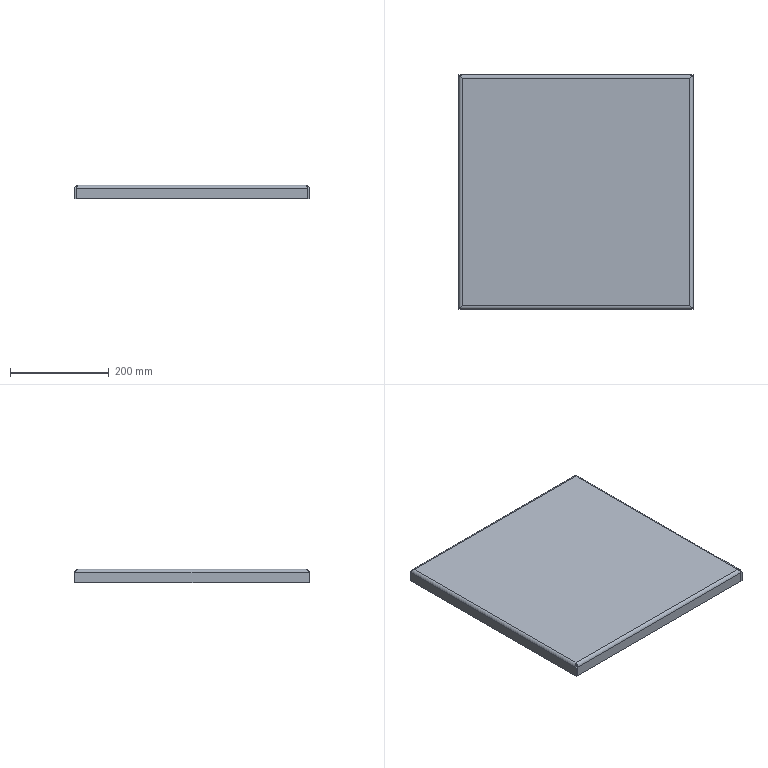Part | SolidWorks | features CornerFeat 4, FlatPattern 1, SMBaseFlange 1, SMMiteredFlange 1, SheetMetal 1 | 1 solid | 38 faces | box 476 x 476 x 28 mm | volume 807964 mm3 | plane 22 | spline 8 | cylinder 8 | commonest cylinder face diameters 8 x4 14 x4
STEP:
#1=CARTESIAN_POINT('',(231.,-231.,0.));
#2=VERTEX_POINT('',#1);
#3=CARTESIAN_POINT('',(-231.,-231.,0.));
#4=VERTEX_POINT('',#3);
#5=CARTESIAN_POINT('',(2585.,-231.,0.));
#6=DIRECTION('',(-1.,0.,0.));
#7=VECTOR('',#6,1000.);
#8=LINE('',#5,#7);
#9=EDGE_CURVE('',#2,#4,#8,.T.);
#10=ORIENTED_EDGE('',*,*,#9,.F.);
#11=CARTESIAN_POINT('',(231.,231.,0.));
#12=VERTEX_POINT('',#11);
#13=CARTESIAN_POINT('',(231.,2585.,0.));
#14=DIRECTION('',(0.,-1.,0.));
#15=VECTOR('',#14,1000.);
#16=LINE('',#13,#15);
#17=EDGE_CURVE('',#12,#2,#16,.T.);
#18=ORIENTED_EDGE('',*,*,#17,.F.);
#19=CARTESIAN_POINT('',(-231.,231.,0.));
#20=VERTEX_POINT('',#19);
#21=CARTESIAN_POINT('',(-2585.,231.,0.));
#22=DIRECTION('',(1.,0.,0.));
#23=VECTOR('',#22,1000.);
#24=LINE('',#21,#23);
#25=EDGE_CURVE('',#20,#12,#24,.T.);
#26=ORIENTED_EDGE('',*,*,#25,.F.);
#27=CARTESIAN_POINT('',(-231.,-2585.,0.));
#28=DIRECTION('',(0.,1.,0.));
#29=VECTOR('',#28,1000.);
#30=LINE('',#27,#29);
#31=EDGE_CURVE('',#4,#20,#30,.T.);
#32=ORIENTED_EDGE('',*,*,#31,.F.);
#33=EDGE_LOOP('',(#10,#18,#26,#32));
#34=FACE_OUTER_BOUND('',#33,.T.);
#35=CARTESIAN_POINT('',(0.,0.,0.));
#36=DIRECTION('',(0.,0.,-1.));
#37=DIRECTION('',(-1.,0.,0.));
#38=AXIS2_PLACEMENT_3D('',#35,#36,#37);
#39=PLANE('',#38);
#40=ADVANCED_FACE('',(#34),#39,.F.);
#41=CARTESIAN_POINT('',(231.,231.,-3.));
#42=VERTEX_POINT('',#41);
#43=CARTESIAN_POINT('',(231.,-231.,-3.));
#44=VERTEX_POINT('',#43);
#45=CARTESIAN_POINT('',(231.,2585.,-3.));
#46=DIRECTION('',(0.,-1.,0.));
#47=VECTOR('',#46,1000.);
#48=LINE('',#45,#47);
#49=EDGE_CURVE('',#42,#44,#48,.T.);
#50=ORIENTED_EDGE('',*,*,#49,.T.);
#51=CARTESIAN_POINT('',(-231.,-231.,-3.));
#52=VERTEX_POINT('',#51);
#53=CARTESIAN_POINT('',(2585.,-231.,-3.));
#54=DIRECTION('',(-1.,0.,0.));
#55=VECTOR('',#54,1000.);
#56=LINE('',#53,#55);
#57=EDGE_CURVE('',#44,#52,#56,.T.);
#58=ORIENTED_EDGE('',*,*,#57,.T.);
#59=CARTESIAN_POINT('',(-231.,231.,-3.));
#60=VERTEX_POINT('',#59);
#61=CARTESIAN_POINT('',(-231.,-2585.,-3.));
#62=DIRECTION('',(0.,1.,0.));
#63=VECTOR('',#62,1000.);
#64=LINE('',#61,#63);
#65=EDGE_CURVE('',#52,#60,#64,.T.);
#66=ORIENTED_EDGE('',*,*,#65,.T.);
#67=CARTESIAN_POINT('',(-2585.,231.,-3.));
#68=DIRECTION('',(1.,0.,0.));
#69=VECTOR('',#68,1000.);
#70=LINE('',#67,#69);
#71=EDGE_CURVE('',#60,#42,#70,.T.);
#72=ORIENTED_EDGE('',*,*,#71,.T.);
#73=EDGE_LOOP('',(#50,#58,#66,#72));
#74=FACE_OUTER_BOUND('',#73,.T.);
#75=CARTESIAN_POINT('',(0.,0.,-3.));
#76=DIRECTION('',(0.,0.,-1.));
#77=DIRECTION('',(-1.,0.,0.));
#78=AXIS2_PLACEMENT_3D('',#75,#76,#77);
#79=PLANE('',#78);
#80=ADVANCED_FACE('',(#74),#79,.T.);
#81=CARTESIAN_POINT('',(234.9,235.,-7.));
#82=VERTEX_POINT('',#81);
#83=CARTESIAN_POINT('',(234.9,238.,-7.));
#84=VERTEX_POINT('',#83);
#85=CARTESIAN_POINT('',(234.9,235.,-7.));
#86=CARTESIAN_POINT('',(234.9,238.,-7.));
#87=B_SPLINE_CURVE_WITH_KNOTS('',1,(#85,#86),.UNSPECIFIED.,.F.,.F.,(2,2),(0.,1.),.UNSPECIFIED.);
#88=EDGE_CURVE('',#82,#84,#87,.T.);
#89=ORIENTED_EDGE('',*,*,#88,.T.);
#90=CARTESIAN_POINT('',(234.9,238.,-7.));
#91=CARTESIAN_POINT('',(234.736,238.,-6.538));
#92=CARTESIAN_POINT('',(234.575,237.955,-6.083));
#93=CARTESIAN_POINT('',(234.332,237.821,-5.412));
#94=CARTESIAN_POINT('',(234.251,237.766,-5.191));
#95=CARTESIAN_POINT('',(234.089,237.633,-4.752));
#96=CARTESIAN_POINT('',(234.007,237.555,-4.534));
#97=CARTESIAN_POINT('',(233.762,237.291,-3.897));
#98=CARTESIAN_POINT('',(233.601,237.076,-3.494));
#99=CARTESIAN_POINT('',(233.358,236.696,-2.925));
#100=CARTESIAN_POINT('',(233.277,236.56,-2.741));
#101=CARTESIAN_POINT('',(233.114,236.268,-2.385));
#102=CARTESIAN_POINT('',(233.032,236.113,-2.213));
#103=CARTESIAN_POINT('',(232.788,235.627,-1.727));
#104=CARTESIAN_POINT('',(232.627,235.275,-1.438));
#105=CARTESIAN_POINT('',(232.303,234.515,-0.9293));
#106=CARTESIAN_POINT('',(232.138,234.104,-0.7093));
#107=CARTESIAN_POINT('',(231.814,233.26,-0.3593));
#108=CARTESIAN_POINT('',(231.653,232.824,-0.2263));
#109=CARTESIAN_POINT('',(231.328,231.925,-0.04623));
#110=CARTESIAN_POINT('',(231.164,231.462,0.));
#111=CARTESIAN_POINT('',(231.,231.,0.));
#112=B_SPLINE_CURVE_WITH_KNOTS('',3,(#90,#91,#92,#93,#94,#95,#96,#97,#98,#99,#100,#101,#102,#103,#104,#105,#106,#107,#108,#109,#110,#111),.UNSPECIFIED.,.F.,.F.,(4,2,2,2,2,2,2,2,2,2,4),(0.,0.00145,0.002176,0.002901,0.004351,0.005076,0.005802,0.007252,0.008702,0.01015,0.0116),.UNSPECIFIED.);
#113=EDGE_CURVE('',#84,#12,#112,.T.);
#114=ORIENTED_EDGE('',*,*,#113,.T.);
#115=CARTESIAN_POINT('',(231.,231.,-3.));
#116=CARTESIAN_POINT('',(231.,231.,0.));
#117=B_SPLINE_CURVE_WITH_KNOTS('',1,(#115,#116),.UNSPECIFIED.,.F.,.F.,(2,2),(0.,1.),.UNSPECIFIED.);
#118=EDGE_CURVE('',#42,#12,#117,.T.);
#119=ORIENTED_EDGE('',*,*,#118,.F.);
#120=CARTESIAN_POINT('',(234.9,235.,-7.));
#121=CARTESIAN_POINT('',(234.736,235.,-6.736));
#122=CARTESIAN_POINT('',(234.574,234.974,-6.475));
#123=CARTESIAN_POINT('',(234.249,234.872,-5.962));
#124=CARTESIAN_POINT('',(234.085,234.794,-5.707));
#125=CARTESIAN_POINT('',(233.76,234.594,-5.224));
#126=CARTESIAN_POINT('',(233.599,234.47,-4.994));
#127=CARTESIAN_POINT('',(233.275,234.181,-4.56));
#128=CARTESIAN_POINT('',(233.111,234.012,-4.355));
#129=CARTESIAN_POINT('',(232.786,233.641,-3.985));
#130=CARTESIAN_POINT('',(232.625,233.44,-3.819));
#131=CARTESIAN_POINT('',(232.301,233.006,-3.53));
#132=CARTESIAN_POINT('',(232.137,232.772,-3.404));
#133=CARTESIAN_POINT('',(231.812,232.288,-3.204));
#134=CARTESIAN_POINT('',(231.651,232.038,-3.128));
#135=CARTESIAN_POINT('',(231.327,231.527,-3.026));
#136=CARTESIAN_POINT('',(231.164,231.264,-3.));
#137=CARTESIAN_POINT('',(231.,231.,-3.));
#138=B_SPLINE_CURVE_WITH_KNOTS('',3,(#120,#121,#122,#123,#124,#125,#126,#127,#128,#129,#130,#131,#132,#133,#134,#135,#136,#137),.UNSPECIFIED.,.F.,.F.,(4,2,2,2,2,2,2,2,4),(0.,0.0009235,0.001847,0.00277,0.003694,0.004617,0.005541,0.006464,0.007388),.UNSPECIFIED.);
#139=EDGE_CURVE('',#82,#42,#138,.T.);
#140=ORIENTED_EDGE('',*,*,#139,.F.);
#141=EDGE_LOOP('',(#89,#114,#119,#140));
#142=FACE_OUTER_BOUND('',#141,.T.);
#143=CARTESIAN_POINT('',(234.9,238.03,-7.));
#144=CARTESIAN_POINT('',(234.575,238.03,-6.08));
#145=CARTESIAN_POINT('',(234.25,237.847,-5.16));
#146=CARTESIAN_POINT('',(233.6,237.143,-3.459));
#147=CARTESIAN_POINT('',(233.275,236.622,-2.68));
#148=CARTESIAN_POINT('',(232.625,235.32,-1.378));
#149=CARTESIAN_POINT('',(232.3,234.541,-0.857));
#150=CARTESIAN_POINT('',(231.65,232.84,-0.1527));
#151=CARTESIAN_POINT('',(231.325,231.92,0.0303));
#152=CARTESIAN_POINT('',(231.,231.,0.0303));
#153=CARTESIAN_POINT('',(234.9,238.,-7.));
#154=CARTESIAN_POINT('',(234.575,238.,-6.084));
#155=CARTESIAN_POINT('',(234.25,237.818,-5.168));
#156=CARTESIAN_POINT('',(233.6,237.117,-3.475));
#157=CARTESIAN_POINT('',(233.275,236.598,-2.698));
#158=CARTESIAN_POINT('',(232.625,235.302,-1.402));
#159=CARTESIAN_POINT('',(232.3,234.525,-0.8835));
#160=CARTESIAN_POINT('',(231.65,232.832,-0.1822));
#161=CARTESIAN_POINT('',(231.325,231.916,0.));
#162=CARTESIAN_POINT('',(231.,231.,0.));
#163=CARTESIAN_POINT('',(234.9,235.,-7.));
#164=CARTESIAN_POINT('',(234.575,235.,-6.476));
#165=CARTESIAN_POINT('',(234.25,234.896,-5.953));
#166=CARTESIAN_POINT('',(233.6,234.495,-4.986));
#167=CARTESIAN_POINT('',(233.275,234.199,-4.542));
#168=CARTESIAN_POINT('',(232.625,233.458,-3.801));
#169=CARTESIAN_POINT('',(232.3,233.014,-3.505));
#170=CARTESIAN_POINT('',(231.65,232.047,-3.104));
#171=CARTESIAN_POINT('',(231.325,231.524,-3.));
#172=CARTESIAN_POINT('',(231.,231.,-3.));
#173=CARTESIAN_POINT('',(234.9,234.97,-7.));
#174=CARTESIAN_POINT('',(234.575,234.97,-6.48));
#175=CARTESIAN_POINT('',(234.25,234.867,-5.961));
#176=CARTESIAN_POINT('',(233.6,234.469,-5.001));
#177=CARTESIAN_POINT('',(233.275,234.175,-4.56));
#178=CARTESIAN_POINT('',(232.625,233.44,-3.825));
#179=CARTESIAN_POINT('',(232.3,232.999,-3.531));
#180=CARTESIAN_POINT('',(231.65,232.039,-3.133));
#181=CARTESIAN_POINT('',(231.325,231.52,-3.03));
#182=CARTESIAN_POINT('',(231.,231.,-3.03));
#183=B_SPLINE_SURFACE_WITH_KNOTS('',1,3,((#143,#144,#145,#146,#147,#148,#149,#150,#151,#152),(#153,#154,#155,#156,#157,#158,#159,#160,#161,#162),(#163,#164,#165,#166,#167,#168,#169,#170,#171,#172),(#173,#174,#175,#176,#177,#178,#179,#180,#181,#182)),.UNSPECIFIED.,.F.,.F.,.F.,(2,1,1,2),(4,2,2,2,4),(-0.0101,0.,1.,1.01),(0.,0.25,0.5,0.75,1.),.UNSPECIFIED.);
#184=ADVANCED_FACE('',(#142),#183,.F.);
#185=CARTESIAN_POINT('',(-234.9,238.,-7.));
#186=VERTEX_POINT('',#185);
#187=CARTESIAN_POINT('',(-231.,231.,0.));
#188=CARTESIAN_POINT('',(-231.164,231.462,0.));
#189=CARTESIAN_POINT('',(-231.325,231.917,-0.04539));
#190=CARTESIAN_POINT('',(-231.568,232.588,-0.1786));
#191=CARTESIAN_POINT('',(-231.649,232.809,-0.2339));
#192=CARTESIAN_POINT('',(-231.811,233.248,-0.3668));
#193=CARTESIAN_POINT('',(-231.893,233.466,-0.4447));
#194=CARTESIAN_POINT('',(-232.138,234.103,-0.7087));
#195=CARTESIAN_POINT('',(-232.299,234.506,-0.924));
#196=CARTESIAN_POINT('',(-232.542,235.075,-1.304));
#197=CARTESIAN_POINT('',(-232.623,235.259,-1.44));
#198=CARTESIAN_POINT('',(-232.786,235.615,-1.732));
#199=CARTESIAN_POINT('',(-232.868,235.787,-1.887));
#200=CARTESIAN_POINT('',(-233.112,236.273,-2.373));
#201=CARTESIAN_POINT('',(-233.273,236.562,-2.725));
#202=CARTESIAN_POINT('',(-233.597,237.071,-3.485));
#203=CARTESIAN_POINT('',(-233.762,237.291,-3.896));
#204=CARTESIAN_POINT('',(-234.086,237.641,-4.74));
#205=CARTESIAN_POINT('',(-234.247,237.774,-5.176));
#206=CARTESIAN_POINT('',(-234.572,237.954,-6.075));
#207=CARTESIAN_POINT('',(-234.736,238.,-6.538));
#208=CARTESIAN_POINT('',(-234.9,238.,-7.));
#209=B_SPLINE_CURVE_WITH_KNOTS('',3,(#187,#188,#189,#190,#191,#192,#193,#194,#195,#196,#197,#198,#199,#200,#201,#202,#203,#204,#205,#206,#207,#208),.UNSPECIFIED.,.F.,.F.,(4,2,2,2,2,2,2,2,2,2,4),(0.,0.00145,0.002176,0.002901,0.004351,0.005076,0.005802,0.007252,0.008702,0.01015,0.0116),.UNSPECIFIED.);
#210=EDGE_CURVE('',#20,#186,#209,.T.);
#211=ORIENTED_EDGE('',*,*,#210,.T.);
#212=CARTESIAN_POINT('',(-234.9,235.,-7.));
#213=VERTEX_POINT('',#212);
#214=CARTESIAN_POINT('',(-234.9,235.,-7.));
#215=CARTESIAN_POINT('',(-234.9,236.,-7.));
#216=CARTESIAN_POINT('',(-234.9,237.,-7.));
#217=CARTESIAN_POINT('',(-234.9,238.,-7.));
#218=B_SPLINE_CURVE_WITH_KNOTS('',3,(#214,#215,#216,#217),.UNSPECIFIED.,.F.,.F.,(4,4),(0.,1.),.UNSPECIFIED.);
#219=EDGE_CURVE('',#213,#186,#218,.T.);
#220=ORIENTED_EDGE('',*,*,#219,.F.);
#221=CARTESIAN_POINT('',(-231.,231.,-3.));
#222=CARTESIAN_POINT('',(-231.164,231.264,-3.));
#223=CARTESIAN_POINT('',(-231.326,231.525,-3.026));
#224=CARTESIAN_POINT('',(-231.651,232.038,-3.128));
#225=CARTESIAN_POINT('',(-231.815,232.292,-3.205));
#226=CARTESIAN_POINT('',(-232.14,232.776,-3.406));
#227=CARTESIAN_POINT('',(-232.301,233.006,-3.53));
#228=CARTESIAN_POINT('',(-232.625,233.44,-3.819));
#229=CARTESIAN_POINT('',(-232.789,233.645,-3.988));
#230=CARTESIAN_POINT('',(-233.114,234.015,-4.359));
#231=CARTESIAN_POINT('',(-233.275,234.181,-4.561));
#232=CARTESIAN_POINT('',(-233.599,234.47,-4.994));
#233=CARTESIAN_POINT('',(-233.763,234.596,-5.228));
#234=CARTESIAN_POINT('',(-234.088,234.796,-5.712));
#235=CARTESIAN_POINT('',(-234.25,234.872,-5.962));
#236=CARTESIAN_POINT('',(-234.573,234.974,-6.473));
#237=CARTESIAN_POINT('',(-234.736,235.,-6.736));
#238=CARTESIAN_POINT('',(-234.9,235.,-7.));
#239=B_SPLINE_CURVE_WITH_KNOTS('',3,(#221,#222,#223,#224,#225,#226,#227,#228,#229,#230,#231,#232,#233,#234,#235,#236,#237,#238),.UNSPECIFIED.,.F.,.F.,(4,2,2,2,2,2,2,2,4),(0.,0.0009233,0.001847,0.00277,0.003693,0.004617,0.00554,0.006463,0.007387),.UNSPECIFIED.);
#240=EDGE_CURVE('',#60,#213,#239,.T.);
#241=ORIENTED_EDGE('',*,*,#240,.F.);
#242=CARTESIAN_POINT('',(-231.,231.,-3.));
#243=CARTESIAN_POINT('',(-231.,231.,0.));
#244=B_SPLINE_CURVE_WITH_KNOTS('',1,(#242,#243),.UNSPECIFIED.,.F.,.F.,(2,2),(0.,1.),.UNSPECIFIED.);
#245=EDGE_CURVE('',#60,#20,#244,.T.);
#246=ORIENTED_EDGE('',*,*,#245,.T.);
#247=EDGE_LOOP('',(#211,#220,#241,#246));
#248=FACE_OUTER_BOUND('',#247,.T.);
#249=CARTESIAN_POINT('',(-231.,231.,0.03));
#250=CARTESIAN_POINT('',(-231.325,231.92,0.03));
#251=CARTESIAN_POINT('',(-231.65,232.84,-0.153));
#252=CARTESIAN_POINT('',(-232.3,234.54,-0.8573));
#253=CARTESIAN_POINT('',(-232.625,235.32,-1.378));
#254=CARTESIAN_POINT('',(-233.275,236.622,-2.68));
#255=CARTESIAN_POINT('',(-233.6,237.143,-3.46));
#256=CARTESIAN_POINT('',(-234.25,237.847,-5.16));
#257=CARTESIAN_POINT('',(-234.575,238.03,-6.08));
#258=CARTESIAN_POINT('',(-234.9,238.03,-7.));
#259=CARTESIAN_POINT('',(-231.,231.,0.));
#260=CARTESIAN_POINT('',(-231.325,231.916,0.));
#261=CARTESIAN_POINT('',(-231.65,232.832,-0.1822));
#262=CARTESIAN_POINT('',(-232.3,234.525,-0.8835));
#263=CARTESIAN_POINT('',(-232.625,235.302,-1.402));
#264=CARTESIAN_POINT('',(-233.275,236.598,-2.698));
#265=CARTESIAN_POINT('',(-233.6,237.117,-3.475));
#266=CARTESIAN_POINT('',(-234.25,237.818,-5.168));
#267=CARTESIAN_POINT('',(-234.575,238.,-6.084));
#268=CARTESIAN_POINT('',(-234.9,238.,-7.));
#269=CARTESIAN_POINT('',(-231.,231.,-3.));
#270=CARTESIAN_POINT('',(-231.325,231.524,-3.));
#271=CARTESIAN_POINT('',(-231.65,232.047,-3.104));
#272=CARTESIAN_POINT('',(-232.3,233.014,-3.505));
#273=CARTESIAN_POINT('',(-232.625,233.458,-3.801));
#274=CARTESIAN_POINT('',(-233.275,234.199,-4.542));
#275=CARTESIAN_POINT('',(-233.6,234.495,-4.986));
#276=CARTESIAN_POINT('',(-234.25,234.896,-5.953));
#277=CARTESIAN_POINT('',(-234.575,235.,-6.476));
#278=CARTESIAN_POINT('',(-234.9,235.,-7.));
#279=CARTESIAN_POINT('',(-231.,231.,-3.03));
#280=CARTESIAN_POINT('',(-231.325,231.52,-3.03));
#281=CARTESIAN_POINT('',(-231.65,232.039,-3.134));
#282=CARTESIAN_POINT('',(-232.3,232.999,-3.531));
#283=CARTESIAN_POINT('',(-232.625,233.44,-3.826));
#284=CARTESIAN_POINT('',(-233.275,234.174,-4.56));
#285=CARTESIAN_POINT('',(-233.6,234.469,-5.001));
#286=CARTESIAN_POINT('',(-234.25,234.866,-5.961));
#287=CARTESIAN_POINT('',(-234.575,234.97,-6.48));
#288=CARTESIAN_POINT('',(-234.9,234.97,-7.));
#289=B_SPLINE_SURFACE_WITH_KNOTS('',1,3,((#249,#250,#251,#252,#253,#254,#255,#256,#257,#258),(#259,#260,#261,#262,#263,#264,#265,#266,#267,#268),(#269,#270,#271,#272,#273,#274,#275,#276,#277,#278),(#279,#280,#281,#282,#283,#284,#285,#286,#287,#288)),.UNSPECIFIED.,.F.,.F.,.F.,(2,1,1,2),(4,2,2,2,4),(-0.01,0.,1.,1.01),(0.,0.25,0.5,0.75,1.),.UNSPECIFIED.);
#290=ADVANCED_FACE('',(#248),#289,.F.);
#291=ORIENTED_EDGE('',*,*,#71,.F.);
#292=ORIENTED_EDGE('',*,*,#240,.T.);
#293=CARTESIAN_POINT('',(-2585.,235.,-7.));
#294=DIRECTION('',(1.,0.,0.));
#295=VECTOR('',#294,1000.);
#296=LINE('',#293,#295);
#297=EDGE_CURVE('',#213,#82,#296,.T.);
#298=ORIENTED_EDGE('',*,*,#297,.T.);
#299=ORIENTED_EDGE('',*,*,#139,.T.);
#300=EDGE_LOOP('',(#291,#292,#298,#299));
#301=FACE_OUTER_BOUND('',#300,.T.);
#302=CARTESIAN_POINT('',(-469.889,231.,-7.));
#303=DIRECTION('',(1.,0.,0.));
#304=DIRECTION('',(0.,1.,0.));
#305=AXIS2_PLACEMENT_3D('',#302,#303,#304);
#306=CYLINDRICAL_SURFACE('',#305,4.);
#307=ADVANCED_FACE('',(#301),#306,.F.);
#308=ORIENTED_EDGE('',*,*,#25,.T.);
#309=ORIENTED_EDGE('',*,*,#113,.F.);
#310=CARTESIAN_POINT('',(-2585.,238.,-7.));
#311=DIRECTION('',(1.,0.,0.));
#312=VECTOR('',#311,1000.);
#313=LINE('',#310,#312);
#314=EDGE_CURVE('',#186,#84,#313,.T.);
#315=ORIENTED_EDGE('',*,*,#314,.F.);
#316=ORIENTED_EDGE('',*,*,#210,.F.);
#317=EDGE_LOOP('',(#308,#309,#315,#316));
#318=FACE_OUTER_BOUND('',#317,.T.);
#319=CARTESIAN_POINT('',(-469.889,231.,-7.));
#320=DIRECTION('',(1.,0.,0.));
#321=DIRECTION('',(0.,1.,0.));
#322=AXIS2_PLACEMENT_3D('',#319,#320,#321);
#323=CYLINDRICAL_SURFACE('',#322,7.);
#324=ADVANCED_FACE('',(#318),#323,.T.);
#325=CARTESIAN_POINT('',(-234.9,238.,-28.));
#326=VERTEX_POINT('',#325);
#327=CARTESIAN_POINT('',(234.9,238.,-28.));
#328=VERTEX_POINT('',#327);
#329=CARTESIAN_POINT('',(-2585.,238.,-28.));
#330=DIRECTION('',(1.,0.,0.));
#331=VECTOR('',#330,1000.);
#332=LINE('',#329,#331);
#333=EDGE_CURVE('',#326,#328,#332,.T.);
#334=ORIENTED_EDGE('',*,*,#333,.T.);
#335=CARTESIAN_POINT('',(234.9,235.,-28.));
#336=VERTEX_POINT('',#335);
#337=CARTESIAN_POINT('',(234.9,235.,-28.));
#338=DIRECTION('',(0.,1.,0.));
#339=VECTOR('',#338,1000.);
#340=LINE('',#337,#339);
#341=EDGE_CURVE('',#336,#328,#340,.T.);
#342=ORIENTED_EDGE('',*,*,#341,.F.);
#343=CARTESIAN_POINT('',(-234.9,235.,-28.));
#344=VERTEX_POINT('',#343);
#345=CARTESIAN_POINT('',(-2585.,235.,-28.));
#346=DIRECTION('',(1.,0.,0.));
#347=VECTOR('',#346,1000.);
#348=LINE('',#345,#347);
#349=EDGE_CURVE('',#344,#336,#348,.T.);
#350=ORIENTED_EDGE('',*,*,#349,.F.);
#351=CARTESIAN_POINT('',(-234.9,235.,-28.));
#352=DIRECTION('',(0.,1.,0.));
#353=VECTOR('',#352,1000.);
#354=LINE('',#351,#353);
#355=EDGE_CURVE('',#344,#326,#354,.T.);
#356=ORIENTED_EDGE('',*,*,#355,.T.);
#357=EDGE_LOOP('',(#334,#342,#350,#356));
#358=FACE_OUTER_BOUND('',#357,.T.);
#359=CARTESIAN_POINT('',(-2585.,235.,-28.));
#360=DIRECTION('',(0.,0.,-1.));
#361=DIRECTION('',(-1.,0.,0.));
#362=AXIS2_PLACEMENT_3D('',#359,#360,#361);
#363=PLANE('',#362);
#364=ADVANCED_FACE('',(#358),#363,.T.);
#365=ORIENTED_EDGE('',*,*,#297,.F.);
#366=CARTESIAN_POINT('',(-234.9,235.,-7.));
#367=DIRECTION('',(0.,0.,-1.));
#368=VECTOR('',#367,1000.);
#369=LINE('',#366,#368);
#370=EDGE_CURVE('',#213,#344,#369,.T.);
#371=ORIENTED_EDGE('',*,*,#370,.T.);
#372=ORIENTED_EDGE('',*,*,#349,.T.);
#373=CARTESIAN_POINT('',(234.9,235.,-7.));
#374=DIRECTION('',(0.,0.,-1.));
#375=VECTOR('',#374,1000.);
#376=LINE('',#373,#375);
#377=EDGE_CURVE('',#82,#336,#376,.T.);
#378=ORIENTED_EDGE('',*,*,#377,.F.);
#379=EDGE_LOOP('',(#365,#371,#372,#378));
#380=FACE_OUTER_BOUND('',#379,.T.);
#381=CARTESIAN_POINT('',(-2585.,235.,-28.));
#382=DIRECTION('',(0.,1.,0.));
#383=DIRECTION('',(-1.,0.,0.));
#384=AXIS2_PLACEMENT_3D('',#381,#382,#383);
#385=PLANE('',#384);
#386=ADVANCED_FACE('',(#380),#385,.F.);
#387=CARTESIAN_POINT('',(-234.9,238.,-7.));
#388=DIRECTION('',(0.,0.,-1.));
#389=VECTOR('',#388,1000.);
#390=LINE('',#387,#389);
#391=EDGE_CURVE('',#186,#326,#390,.T.);
#392=ORIENTED_EDGE('',*,*,#391,.T.);
#393=ORIENTED_EDGE('',*,*,#355,.F.);
#394=ORIENTED_EDGE('',*,*,#370,.F.);
#395=ORIENTED_EDGE('',*,*,#219,.T.);
#396=EDGE_LOOP('',(#392,#393,#394,#395));
#397=FACE_OUTER_BOUND('',#396,.T.);
#398=CARTESIAN_POINT('',(-234.9,235.,-7.));
#399=DIRECTION('',(1.,0.,0.));
#400=DIRECTION('',(0.,0.,1.));
#401=AXIS2_PLACEMENT_3D('',#398,#399,#400);
#402=PLANE('',#401);
#403=ADVANCED_FACE('',(#397),#402,.F.);
#404=ORIENTED_EDGE('',*,*,#314,.T.);
#405=CARTESIAN_POINT('',(234.9,238.,-7.));
#406=DIRECTION('',(0.,0.,-1.));
#407=VECTOR('',#406,1000.);
#408=LINE('',#405,#407);
#409=EDGE_CURVE('',#84,#328,#408,.T.);
#410=ORIENTED_EDGE('',*,*,#409,.T.);
#411=ORIENTED_EDGE('',*,*,#333,.F.);
#412=ORIENTED_EDGE('',*,*,#391,.F.);
#413=EDGE_LOOP('',(#404,#410,#411,#412));
#414=FACE_OUTER_BOUND('',#413,.T.);
#415=CARTESIAN_POINT('',(-2585.,238.,-28.));
#416=DIRECTION('',(0.,1.,0.));
#417=DIRECTION('',(-1.,0.,0.));
#418=AXIS2_PLACEMENT_3D('',#415,#416,#417);
#419=PLANE('',#418);
#420=ADVANCED_FACE('',(#414),#419,.T.);
#421=ORIENTED_EDGE('',*,*,#409,.F.);
#422=ORIENTED_EDGE('',*,*,#88,.F.);
#423=ORIENTED_EDGE('',*,*,#377,.T.);
#424=ORIENTED_EDGE('',*,*,#341,.T.);
#425=EDGE_LOOP('',(#421,#422,#423,#424));
#426=FACE_OUTER_BOUND('',#425,.T.);
#427=CARTESIAN_POINT('',(234.9,235.,-7.));
#428=DIRECTION('',(1.,0.,0.));
#429=DIRECTION('',(0.,0.,-1.));
#430=AXIS2_PLACEMENT_3D('',#427,#428,#429);
#431=PLANE('',#430);
#432=ADVANCED_FACE('',(#426),#431,.T.);
#433=CARTESIAN_POINT('',(-238.,-238.,-28.));
#434=VERTEX_POINT('',#433);
#435=CARTESIAN_POINT('',(-238.,238.,-28.));
#436=VERTEX_POINT('',#435);
#437=CARTESIAN_POINT('',(-238.,-2585.,-28.));
#438=DIRECTION('',(0.,1.,0.));
#439=VECTOR('',#438,1000.);
#440=LINE('',#437,#439);
#441=EDGE_CURVE('',#434,#436,#440,.T.);
#442=ORIENTED_EDGE('',*,*,#441,.T.);
#443=CARTESIAN_POINT('',(-235.,238.,-28.));
#444=VERTEX_POINT('',#443);
#445=CARTESIAN_POINT('',(-238.,238.,-28.));
#446=DIRECTION('',(1.,0.,0.));
#447=VECTOR('',#446,1000.);
#448=LINE('',#445,#447);
#449=EDGE_CURVE('',#436,#444,#448,.T.);
#450=ORIENTED_EDGE('',*,*,#449,.T.);
#451=CARTESIAN_POINT('',(-235.,-238.,-28.));
#452=VERTEX_POINT('',#451);
#453=CARTESIAN_POINT('',(-235.,-2585.,-28.));
#454=DIRECTION('',(0.,1.,0.));
#455=VECTOR('',#454,1000.);
#456=LINE('',#453,#455);
#457=EDGE_CURVE('',#452,#444,#456,.T.);
#458=ORIENTED_EDGE('',*,*,#457,.F.);
#459=CARTESIAN_POINT('',(-238.,-238.,-28.));
#460=DIRECTION('',(1.,0.,0.));
#461=VECTOR('',#460,1000.);
#462=LINE('',#459,#461);
#463=EDGE_CURVE('',#434,#452,#462,.T.);
#464=ORIENTED_EDGE('',*,*,#463,.F.);
#465=EDGE_LOOP('',(#442,#450,#458,#464));
#466=FACE_OUTER_BOUND('',#465,.T.);
#467=CARTESIAN_POINT('',(-235.,-2585.,-28.));
#468=DIRECTION('',(0.,0.,-1.));
#469=DIRECTION('',(0.,-1.,0.));
#470=AXIS2_PLACEMENT_3D('',#467,#468,#469);
#471=PLANE('',#470);
#472=ADVANCED_FACE('',(#466),#471,.T.);
#473=CARTESIAN_POINT('',(-235.,-238.,-7.));
#474=VERTEX_POINT('',#473);
#475=CARTESIAN_POINT('',(-235.,238.,-7.));
#476=VERTEX_POINT('',#475);
#477=CARTESIAN_POINT('',(-235.,-2585.,-7.));
#478=DIRECTION('',(0.,1.,0.));
#479=VECTOR('',#478,1000.);
#480=LINE('',#477,#479);
#481=EDGE_CURVE('',#474,#476,#480,.T.);
#482=ORIENTED_EDGE('',*,*,#481,.F.);
#483=CARTESIAN_POINT('',(-235.,-238.,-7.));
#484=DIRECTION('',(0.,0.,-1.));
#485=VECTOR('',#484,1000.);
#486=LINE('',#483,#485);
#487=EDGE_CURVE('',#474,#452,#486,.T.);
#488=ORIENTED_EDGE('',*,*,#487,.T.);
#489=ORIENTED_EDGE('',*,*,#457,.T.);
#490=CARTESIAN_POINT('',(-235.,238.,-7.));
#491=DIRECTION('',(0.,0.,-1.));
#492=VECTOR('',#491,1000.);
#493=LINE('',#490,#492);
#494=EDGE_CURVE('',#476,#444,#493,.T.);
#495=ORIENTED_EDGE('',*,*,#494,.F.);
#496=EDGE_LOOP('',(#482,#488,#489,#495));
#497=FACE_OUTER_BOUND('',#496,.T.);
#498=CARTESIAN_POINT('',(-235.,-2585.,-28.));
#499=DIRECTION('',(-1.,0.,0.));
#500=DIRECTION('',(0.,-1.,0.));
#501=AXIS2_PLACEMENT_3D('',#498,#499,#500);
#502=PLANE('',#501);
#503=ADVANCED_FACE('',(#497),#502,.F.);
#504=ORIENTED_EDGE('',*,*,#487,.F.);
#505=CARTESIAN_POINT('',(-238.,-238.,-7.));
#506=VERTEX_POINT('',#505);
#507=CARTESIAN_POINT('',(-238.,-238.,-7.));
#508=CARTESIAN_POINT('',(-235.,-238.,-7.));
#509=B_SPLINE_CURVE_WITH_KNOTS('',1,(#507,#508),.UNSPECIFIED.,.F.,.F.,(2,2),(0.,1.),.UNSPECIFIED.);
#510=EDGE_CURVE('',#506,#474,#509,.T.);
#511=ORIENTED_EDGE('',*,*,#510,.F.);
#512=CARTESIAN_POINT('',(-238.,-238.,-7.));
#513=DIRECTION('',(0.,0.,-1.));
#514=VECTOR('',#513,1000.);
#515=LINE('',#512,#514);
#516=EDGE_CURVE('',#506,#434,#515,.T.);
#517=ORIENTED_EDGE('',*,*,#516,.T.);
#518=ORIENTED_EDGE('',*,*,#463,.T.);
#519=EDGE_LOOP('',(#504,#511,#517,#518));
#520=FACE_OUTER_BOUND('',#519,.T.);
#521=CARTESIAN_POINT('',(-238.,-238.,-7.));
#522=DIRECTION('',(0.,-1.,0.));
#523=DIRECTION('',(0.,0.,-1.));
#524=AXIS2_PLACEMENT_3D('',#521,#522,#523);
#525=PLANE('',#524);
#526=ADVANCED_FACE('',(#520),#525,.T.);
#527=CARTESIAN_POINT('',(-238.,238.,-7.));
#528=VERTEX_POINT('',#527);
#529=CARTESIAN_POINT('',(-238.,-2585.,-7.));
#530=DIRECTION('',(0.,1.,0.));
#531=VECTOR('',#530,1000.);
#532=LINE('',#529,#531);
#533=EDGE_CURVE('',#506,#528,#532,.T.);
#534=ORIENTED_EDGE('',*,*,#533,.T.);
#535=CARTESIAN_POINT('',(-238.,238.,-7.));
#536=DIRECTION('',(0.,0.,-1.));
#537=VECTOR('',#536,1000.);
#538=LINE('',#535,#537);
#539=EDGE_CURVE('',#528,#436,#538,.T.);
#540=ORIENTED_EDGE('',*,*,#539,.T.);
#541=ORIENTED_EDGE('',*,*,#441,.F.);
#542=ORIENTED_EDGE('',*,*,#516,.F.);
#543=EDGE_LOOP('',(#534,#540,#541,#542));
#544=FACE_OUTER_BOUND('',#543,.T.);
#545=CARTESIAN_POINT('',(-238.,-2585.,-28.));
#546=DIRECTION('',(-1.,0.,0.));
#547=DIRECTION('',(0.,-1.,0.));
#548=AXIS2_PLACEMENT_3D('',#545,#546,#547);
#549=PLANE('',#548);
#550=ADVANCED_FACE('',(#544),#549,.T.);
#551=ORIENTED_EDGE('',*,*,#494,.T.);
#552=ORIENTED_EDGE('',*,*,#449,.F.);
#553=ORIENTED_EDGE('',*,*,#539,.F.);
#554=CARTESIAN_POINT('',(-238.,238.,-7.));
#555=CARTESIAN_POINT('',(-237.,238.,-7.));
#556=CARTESIAN_POINT('',(-236.,238.,-7.));
#557=CARTESIAN_POINT('',(-235.,238.,-7.));
#558=B_SPLINE_CURVE_WITH_KNOTS('',3,(#554,#555,#556,#557),.UNSPECIFIED.,.F.,.F.,(4,4),(0.,1.),.UNSPECIFIED.);
#559=EDGE_CURVE('',#528,#476,#558,.T.);
#560=ORIENTED_EDGE('',*,*,#559,.T.);
#561=EDGE_LOOP('',(#551,#552,#553,#560));
#562=FACE_OUTER_BOUND('',#561,.T.);
#563=CARTESIAN_POINT('',(-238.,238.,-7.));
#564=DIRECTION('',(0.,-1.,0.));
#565=DIRECTION('',(0.,0.,-1.));
#566=AXIS2_PLACEMENT_3D('',#563,#564,#565);
#567=PLANE('',#566);
#568=ADVANCED_FACE('',(#562),#567,.F.);
#569=ORIENTED_EDGE('',*,*,#559,.F.);
#570=CARTESIAN_POINT('',(-238.,238.,-7.));
#571=CARTESIAN_POINT('',(-238.,237.417,-6.084));
#572=CARTESIAN_POINT('',(-237.818,236.833,-5.168));
#573=CARTESIAN_POINT('',(-237.117,235.667,-3.475));
#574=CARTESIAN_POINT('',(-236.598,235.083,-2.698));
#575=CARTESIAN_POINT('',(-235.302,233.917,-1.402));
#576=CARTESIAN_POINT('',(-234.525,233.333,-0.8835));
#577=CARTESIAN_POINT('',(-232.832,232.167,-0.1822));
#578=CARTESIAN_POINT('',(-231.916,231.583,0.));
#579=CARTESIAN_POINT('',(-231.,231.,0.));
#580=B_SPLINE_CURVE_WITH_KNOTS('',3,(#570,#571,#572,#573,#574,#575,#576,#577,#578,#579),.UNSPECIFIED.,.F.,.F.,(4,2,2,2,4),(0.,0.25,0.5,0.75,1.),.UNSPECIFIED.);
#581=EDGE_CURVE('',#528,#20,#580,.T.);
#582=ORIENTED_EDGE('',*,*,#581,.T.);
#583=ORIENTED_EDGE('',*,*,#245,.F.);
#584=CARTESIAN_POINT('',(-235.,238.,-7.));
#585=CARTESIAN_POINT('',(-235.,237.417,-6.476));
#586=CARTESIAN_POINT('',(-234.896,236.833,-5.953));
#587=CARTESIAN_POINT('',(-234.495,235.667,-4.986));
#588=CARTESIAN_POINT('',(-234.199,235.083,-4.542));
#589=CARTESIAN_POINT('',(-233.458,233.917,-3.801));
#590=CARTESIAN_POINT('',(-233.014,233.333,-3.505));
#591=CARTESIAN_POINT('',(-232.047,232.167,-3.104));
#592=CARTESIAN_POINT('',(-231.524,231.583,-3.));
#593=CARTESIAN_POINT('',(-231.,231.,-3.));
#594=B_SPLINE_CURVE_WITH_KNOTS('',3,(#584,#585,#586,#587,#588,#589,#590,#591,#592,#593),.UNSPECIFIED.,.F.,.F.,(4,2,2,2,4),(0.,0.25,0.5,0.75,1.),.UNSPECIFIED.);
#595=EDGE_CURVE('',#476,#60,#594,.T.);
#596=ORIENTED_EDGE('',*,*,#595,.F.);
#597=EDGE_LOOP('',(#569,#582,#583,#596));
#598=FACE_OUTER_BOUND('',#597,.T.);
#599=CARTESIAN_POINT('',(-238.,238.,-7.));
#600=CARTESIAN_POINT('',(-238.,237.417,-6.084));
#601=CARTESIAN_POINT('',(-237.818,236.833,-5.168));
#602=CARTESIAN_POINT('',(-237.117,235.667,-3.475));
#603=CARTESIAN_POINT('',(-236.598,235.083,-2.698));
#604=CARTESIAN_POINT('',(-235.302,233.917,-1.402));
#605=CARTESIAN_POINT('',(-234.525,233.333,-0.8835));
#606=CARTESIAN_POINT('',(-232.832,232.167,-0.1822));
#607=CARTESIAN_POINT('',(-231.916,231.583,0.));
#608=CARTESIAN_POINT('',(-231.,231.,0.));
#609=CARTESIAN_POINT('',(-235.,238.,-7.));
#610=CARTESIAN_POINT('',(-235.,237.417,-6.476));
#611=CARTESIAN_POINT('',(-234.896,236.833,-5.953));
#612=CARTESIAN_POINT('',(-234.495,235.667,-4.986));
#613=CARTESIAN_POINT('',(-234.199,235.083,-4.542));
#614=CARTESIAN_POINT('',(-233.458,233.917,-3.801));
#615=CARTESIAN_POINT('',(-233.014,233.333,-3.505));
#616=CARTESIAN_POINT('',(-232.047,232.167,-3.104));
#617=CARTESIAN_POINT('',(-231.524,231.583,-3.));
#618=CARTESIAN_POINT('',(-231.,231.,-3.));
#619=B_SPLINE_SURFACE_WITH_KNOTS('',1,3,((#599,#600,#601,#602,#603,#604,#605,#606,#607,#608),(#609,#610,#611,#612,#613,#614,#615,#616,#617,#618)),.UNSPECIFIED.,.F.,.F.,.F.,(2,2),(4,2,2,2,4),(0.,1.),(0.,0.25,0.5,0.75,1.),.UNSPECIFIED.);
#620=ADVANCED_FACE('',(#598),#619,.F.);
#621=CARTESIAN_POINT('',(-231.,-231.,0.));
#622=CARTESIAN_POINT('',(-231.462,-231.294,0.));
#623=CARTESIAN_POINT('',(-231.919,-231.585,-0.04553));
#624=CARTESIAN_POINT('',(-232.591,-232.021,-0.1793));
#625=CARTESIAN_POINT('',(-232.813,-232.167,-0.2349));
#626=CARTESIAN_POINT('',(-233.252,-232.459,-0.368));
#627=CARTESIAN_POINT('',(-233.469,-232.606,-0.446));
#628=CARTESIAN_POINT('',(-234.108,-233.046,-0.711));
#629=CARTESIAN_POINT('',(-234.511,-233.336,-0.9272));
#630=CARTESIAN_POINT('',(-235.269,-233.916,-1.434));
#631=CARTESIAN_POINT('',(-235.625,-234.208,-1.726));
#632=CARTESIAN_POINT('',(-236.278,-234.795,-2.378));
#633=CARTESIAN_POINT('',(-236.568,-235.085,-2.733));
#634=CARTESIAN_POINT('',(-237.074,-235.666,-3.491));
#635=CARTESIAN_POINT('',(-237.291,-235.957,-3.896));
#636=CARTESIAN_POINT('',(-237.821,-236.839,-5.176));
#637=CARTESIAN_POINT('',(-238.,-237.411,-6.075));
#638=CARTESIAN_POINT('',(-238.,-238.,-7.));
#639=B_SPLINE_CURVE_WITH_KNOTS('',3,(#621,#622,#623,#624,#625,#626,#627,#628,#629,#630,#631,#632,#633,#634,#635,#636,#637,#638),.UNSPECIFIED.,.F.,.F.,(4,2,2,2,2,2,2,2,4),(0.,0.001624,0.002437,0.003249,0.004873,0.006498,0.008122,0.009746,0.013),.UNSPECIFIED.);
#640=EDGE_CURVE('',#4,#506,#639,.T.);
#641=ORIENTED_EDGE('',*,*,#640,.T.);
#642=ORIENTED_EDGE('',*,*,#510,.T.);
#643=CARTESIAN_POINT('',(-231.,-231.,-3.));
#644=CARTESIAN_POINT('',(-231.529,-231.589,-3.));
#645=CARTESIAN_POINT('',(-232.046,-232.166,-3.104));
#646=CARTESIAN_POINT('',(-232.772,-233.041,-3.404));
#647=CARTESIAN_POINT('',(-233.007,-233.337,-3.53));
#648=CARTESIAN_POINT('',(-233.443,-233.921,-3.822));
#649=CARTESIAN_POINT('',(-233.645,-234.211,-3.988));
#650=CARTESIAN_POINT('',(-234.014,-234.793,-4.357));
#651=CARTESIAN_POINT('',(-234.181,-235.083,-4.56));
#652=CARTESIAN_POINT('',(-234.473,-235.671,-4.999));
#653=CARTESIAN_POINT('',(-234.598,-235.964,-5.232));
#654=CARTESIAN_POINT('',(-234.896,-236.836,-5.955));
#655=CARTESIAN_POINT('',(-235.,-237.411,-6.471));
#656=CARTESIAN_POINT('',(-235.,-238.,-7.));
#657=B_SPLINE_CURVE_WITH_KNOTS('',3,(#643,#644,#645,#646,#647,#648,#649,#650,#651,#652,#653,#654,#655,#656),.UNSPECIFIED.,.F.,.F.,(4,2,2,2,2,2,4),(0.,0.002342,0.003513,0.004684,0.005856,0.007027,0.009369),.UNSPECIFIED.);
#658=EDGE_CURVE('',#52,#474,#657,.T.);
#659=ORIENTED_EDGE('',*,*,#658,.F.);
#660=CARTESIAN_POINT('',(-231.,-231.,-3.));
#661=CARTESIAN_POINT('',(-231.,-231.,0.));
#662=B_SPLINE_CURVE_WITH_KNOTS('',1,(#660,#661),.UNSPECIFIED.,.F.,.F.,(2,2),(0.,1.),.UNSPECIFIED.);
#663=EDGE_CURVE('',#52,#4,#662,.T.);
#664=ORIENTED_EDGE('',*,*,#663,.T.);
#665=EDGE_LOOP('',(#641,#642,#659,#664));
#666=FACE_OUTER_BOUND('',#665,.T.);
#667=CARTESIAN_POINT('',(-231.,-231.,0.03));
#668=CARTESIAN_POINT('',(-231.92,-231.583,0.03));
#669=CARTESIAN_POINT('',(-232.84,-232.167,-0.153));
#670=CARTESIAN_POINT('',(-234.54,-233.333,-0.8573));
#671=CARTESIAN_POINT('',(-235.32,-233.917,-1.378));
#672=CARTESIAN_POINT('',(-236.622,-235.083,-2.68));
#673=CARTESIAN_POINT('',(-237.143,-235.667,-3.46));
#674=CARTESIAN_POINT('',(-237.847,-236.833,-5.16));
#675=CARTESIAN_POINT('',(-238.03,-237.417,-6.08));
#676=CARTESIAN_POINT('',(-238.03,-238.,-7.));
#677=CARTESIAN_POINT('',(-231.,-231.,0.));
#678=CARTESIAN_POINT('',(-231.916,-231.583,0.));
#679=CARTESIAN_POINT('',(-232.832,-232.167,-0.1822));
#680=CARTESIAN_POINT('',(-234.525,-233.333,-0.8835));
#681=CARTESIAN_POINT('',(-235.302,-233.917,-1.402));
#682=CARTESIAN_POINT('',(-236.598,-235.083,-2.698));
#683=CARTESIAN_POINT('',(-237.117,-235.667,-3.475));
#684=CARTESIAN_POINT('',(-237.818,-236.833,-5.168));
#685=CARTESIAN_POINT('',(-238.,-237.417,-6.084));
#686=CARTESIAN_POINT('',(-238.,-238.,-7.));
#687=CARTESIAN_POINT('',(-231.,-231.,-3.));
#688=CARTESIAN_POINT('',(-231.524,-231.583,-3.));
#689=CARTESIAN_POINT('',(-232.047,-232.167,-3.104));
#690=CARTESIAN_POINT('',(-233.014,-233.333,-3.505));
#691=CARTESIAN_POINT('',(-233.458,-233.917,-3.801));
#692=CARTESIAN_POINT('',(-234.199,-235.083,-4.542));
#693=CARTESIAN_POINT('',(-234.495,-235.667,-4.986));
#694=CARTESIAN_POINT('',(-234.896,-236.833,-5.953));
#695=CARTESIAN_POINT('',(-235.,-237.417,-6.476));
#696=CARTESIAN_POINT('',(-235.,-238.,-7.));
#697=CARTESIAN_POINT('',(-231.,-231.,-3.03));
#698=CARTESIAN_POINT('',(-231.52,-231.583,-3.03));
#699=CARTESIAN_POINT('',(-232.039,-232.167,-3.134));
#700=CARTESIAN_POINT('',(-232.999,-233.333,-3.531));
#701=CARTESIAN_POINT('',(-233.44,-233.917,-3.826));
#702=CARTESIAN_POINT('',(-234.174,-235.083,-4.56));
#703=CARTESIAN_POINT('',(-234.469,-235.667,-5.001));
#704=CARTESIAN_POINT('',(-234.866,-236.833,-5.961));
#705=CARTESIAN_POINT('',(-234.97,-237.417,-6.48));
#706=CARTESIAN_POINT('',(-234.97,-238.,-7.));
#707=B_SPLINE_SURFACE_WITH_KNOTS('',1,3,((#667,#668,#669,#670,#671,#672,#673,#674,#675,#676),(#677,#678,#679,#680,#681,#682,#683,#684,#685,#686),(#687,#688,#689,#690,#691,#692,#693,#694,#695,#696),(#697,#698,#699,#700,#701,#702,#703,#704,#705,#706)),.UNSPECIFIED.,.F.,.F.,.F.,(2,1,1,2),(4,2,2,2,4),(-0.01,0.,1.,1.01),(0.,0.25,0.5,0.75,1.),.UNSPECIFIED.);
#708=ADVANCED_FACE('',(#666),#707,.F.);
#709=ORIENTED_EDGE('',*,*,#65,.F.);
#710=ORIENTED_EDGE('',*,*,#658,.T.);
#711=ORIENTED_EDGE('',*,*,#481,.T.);
#712=ORIENTED_EDGE('',*,*,#595,.T.);
#713=EDGE_LOOP('',(#709,#710,#711,#712));
#714=FACE_OUTER_BOUND('',#713,.T.);
#715=CARTESIAN_POINT('',(-231.,476.088,-7.));
#716=DIRECTION('',(0.,-1.,0.));
#717=DIRECTION('',(1.,0.,0.));
#718=AXIS2_PLACEMENT_3D('',#715,#716,#717);
#719=CYLINDRICAL_SURFACE('',#718,4.);
#720=ADVANCED_FACE('',(#714),#719,.F.);
#721=ORIENTED_EDGE('',*,*,#31,.T.);
#722=ORIENTED_EDGE('',*,*,#581,.F.);
#723=ORIENTED_EDGE('',*,*,#533,.F.);
#724=ORIENTED_EDGE('',*,*,#640,.F.);
#725=EDGE_LOOP('',(#721,#722,#723,#724));
#726=FACE_OUTER_BOUND('',#725,.T.);
#727=CARTESIAN_POINT('',(-231.,476.088,-7.));
#728=DIRECTION('',(0.,-1.,0.));
#729=DIRECTION('',(1.,0.,0.));
#730=AXIS2_PLACEMENT_3D('',#727,#728,#729);
#731=CYLINDRICAL_SURFACE('',#730,7.);
#732=ADVANCED_FACE('',(#726),#731,.T.);
#733=CARTESIAN_POINT('',(238.,238.,-28.));
#734=VERTEX_POINT('',#733);
#735=CARTESIAN_POINT('',(238.,-238.,-28.));
#736=VERTEX_POINT('',#735);
#737=CARTESIAN_POINT('',(238.,2585.,-28.));
#738=DIRECTION('',(0.,-1.,0.));
#739=VECTOR('',#738,1000.);
#740=LINE('',#737,#739);
#741=EDGE_CURVE('',#734,#736,#740,.T.);
#742=ORIENTED_EDGE('',*,*,#741,.T.);
#743=CARTESIAN_POINT('',(235.,-238.,-28.));
#744=VERTEX_POINT('',#743);
#745=CARTESIAN_POINT('',(238.,-238.,-28.));
#746=DIRECTION('',(-1.,0.,0.));
#747=VECTOR('',#746,1000.);
#748=LINE('',#745,#747);
#749=EDGE_CURVE('',#736,#744,#748,.T.);
#750=ORIENTED_EDGE('',*,*,#749,.T.);
#751=CARTESIAN_POINT('',(235.,238.,-28.));
#752=VERTEX_POINT('',#751);
#753=CARTESIAN_POINT('',(235.,2585.,-28.));
#754=DIRECTION('',(0.,-1.,0.));
#755=VECTOR('',#754,1000.);
#756=LINE('',#753,#755);
#757=EDGE_CURVE('',#752,#744,#756,.T.);
#758=ORIENTED_EDGE('',*,*,#757,.F.);
#759=CARTESIAN_POINT('',(238.,238.,-28.));
#760=DIRECTION('',(-1.,0.,0.));
#761=VECTOR('',#760,1000.);
#762=LINE('',#759,#761);
#763=EDGE_CURVE('',#734,#752,#762,.T.);
#764=ORIENTED_EDGE('',*,*,#763,.F.);
#765=EDGE_LOOP('',(#742,#750,#758,#764));
#766=FACE_OUTER_BOUND('',#765,.T.);
#767=CARTESIAN_POINT('',(235.,2585.,-28.));
#768=DIRECTION('',(0.,0.,-1.));
#769=DIRECTION('',(0.,1.,0.));
#770=AXIS2_PLACEMENT_3D('',#767,#768,#769);
#771=PLANE('',#770);
#772=ADVANCED_FACE('',(#766),#771,.T.);
#773=CARTESIAN_POINT('',(235.,238.,-7.));
#774=VERTEX_POINT('',#773);
#775=CARTESIAN_POINT('',(235.,-238.,-7.));
#776=VERTEX_POINT('',#775);
#777=CARTESIAN_POINT('',(235.,2585.,-7.));
#778=DIRECTION('',(0.,-1.,0.));
#779=VECTOR('',#778,1000.);
#780=LINE('',#777,#779);
#781=EDGE_CURVE('',#774,#776,#780,.T.);
#782=ORIENTED_EDGE('',*,*,#781,.F.);
#783=CARTESIAN_POINT('',(235.,238.,-7.));
#784=DIRECTION('',(0.,0.,-1.));
#785=VECTOR('',#784,1000.);
#786=LINE('',#783,#785);
#787=EDGE_CURVE('',#774,#752,#786,.T.);
#788=ORIENTED_EDGE('',*,*,#787,.T.);
#789=ORIENTED_EDGE('',*,*,#757,.T.);
#790=CARTESIAN_POINT('',(235.,-238.,-7.));
#791=DIRECTION('',(0.,0.,-1.));
#792=VECTOR('',#791,1000.);
#793=LINE('',#790,#792);
#794=EDGE_CURVE('',#776,#744,#793,.T.);
#795=ORIENTED_EDGE('',*,*,#794,.F.);
#796=EDGE_LOOP('',(#782,#788,#789,#795));
#797=FACE_OUTER_BOUND('',#796,.T.);
#798=CARTESIAN_POINT('',(235.,2585.,-28.));
#799=DIRECTION('',(1.,0.,0.));
#800=DIRECTION('',(0.,1.,0.));
#801=AXIS2_PLACEMENT_3D('',#798,#799,#800);
#802=PLANE('',#801);
#803=ADVANCED_FACE('',(#797),#802,.F.);
#804=ORIENTED_EDGE('',*,*,#787,.F.);
#805=CARTESIAN_POINT('',(238.,238.,-7.));
#806=VERTEX_POINT('',#805);
#807=CARTESIAN_POINT('',(238.,238.,-7.));
#808=CARTESIAN_POINT('',(235.,238.,-7.));
#809=B_SPLINE_CURVE_WITH_KNOTS('',1,(#807,#808),.UNSPECIFIED.,.F.,.F.,(2,2),(0.,1.),.UNSPECIFIED.);
#810=EDGE_CURVE('',#806,#774,#809,.T.);
#811=ORIENTED_EDGE('',*,*,#810,.F.);
#812=CARTESIAN_POINT('',(238.,238.,-7.));
#813=DIRECTION('',(0.,0.,-1.));
#814=VECTOR('',#813,1000.);
#815=LINE('',#812,#814);
#816=EDGE_CURVE('',#806,#734,#815,.T.);
#817=ORIENTED_EDGE('',*,*,#816,.T.);
#818=ORIENTED_EDGE('',*,*,#763,.T.);
#819=EDGE_LOOP('',(#804,#811,#817,#818));
#820=FACE_OUTER_BOUND('',#819,.T.);
#821=CARTESIAN_POINT('',(238.,238.,-7.));
#822=DIRECTION('',(0.,1.,0.));
#823=DIRECTION('',(-1.,0.,0.));
#824=AXIS2_PLACEMENT_3D('',#821,#822,#823);
#825=PLANE('',#824);
#826=ADVANCED_FACE('',(#820),#825,.T.);
#827=CARTESIAN_POINT('',(238.,-238.,-7.));
#828=VERTEX_POINT('',#827);
#829=CARTESIAN_POINT('',(238.,2585.,-7.));
#830=DIRECTION('',(0.,-1.,0.));
#831=VECTOR('',#830,1000.);
#832=LINE('',#829,#831);
#833=EDGE_CURVE('',#806,#828,#832,.T.);
#834=ORIENTED_EDGE('',*,*,#833,.T.);
#835=CARTESIAN_POINT('',(238.,-238.,-7.));
#836=DIRECTION('',(0.,0.,-1.));
#837=VECTOR('',#836,1000.);
#838=LINE('',#835,#837);
#839=EDGE_CURVE('',#828,#736,#838,.T.);
#840=ORIENTED_EDGE('',*,*,#839,.T.);
#841=ORIENTED_EDGE('',*,*,#741,.F.);
#842=ORIENTED_EDGE('',*,*,#816,.F.);
#843=EDGE_LOOP('',(#834,#840,#841,#842));
#844=FACE_OUTER_BOUND('',#843,.T.);
#845=CARTESIAN_POINT('',(238.,2585.,-28.));
#846=DIRECTION('',(1.,0.,0.));
#847=DIRECTION('',(0.,1.,0.));
#848=AXIS2_PLACEMENT_3D('',#845,#846,#847);
#849=PLANE('',#848);
#850=ADVANCED_FACE('',(#844),#849,.T.);
#851=ORIENTED_EDGE('',*,*,#794,.T.);
#852=ORIENTED_EDGE('',*,*,#749,.F.);
#853=ORIENTED_EDGE('',*,*,#839,.F.);
#854=CARTESIAN_POINT('',(238.,-238.,-7.));
#855=CARTESIAN_POINT('',(237.,-238.,-7.));
#856=CARTESIAN_POINT('',(236.,-238.,-7.));
#857=CARTESIAN_POINT('',(235.,-238.,-7.));
#858=B_SPLINE_CURVE_WITH_KNOTS('',3,(#854,#855,#856,#857),.UNSPECIFIED.,.F.,.F.,(4,4),(0.,1.),.UNSPECIFIED.);
#859=EDGE_CURVE('',#828,#776,#858,.T.);
#860=ORIENTED_EDGE('',*,*,#859,.T.);
#861=EDGE_LOOP('',(#851,#852,#853,#860));
#862=FACE_OUTER_BOUND('',#861,.T.);
#863=CARTESIAN_POINT('',(238.,-238.,-7.));
#864=DIRECTION('',(0.,1.,0.));
#865=DIRECTION('',(-1.,0.,0.));
#866=AXIS2_PLACEMENT_3D('',#863,#864,#865);
#867=PLANE('',#866);
#868=ADVANCED_FACE('',(#862),#867,.F.);
#869=ORIENTED_EDGE('',*,*,#859,.F.);
#870=CARTESIAN_POINT('',(238.,-238.,-7.));
#871=CARTESIAN_POINT('',(238.,-237.706,-6.538));
#872=CARTESIAN_POINT('',(237.954,-237.415,-6.081));
#873=CARTESIAN_POINT('',(237.776,-236.834,-5.186));
#874=CARTESIAN_POINT('',(237.643,-236.542,-4.744));
#875=CARTESIAN_POINT('',(237.289,-235.954,-3.892));
#876=CARTESIAN_POINT('',(237.073,-235.664,-3.489));
#877=CARTESIAN_POINT('',(236.566,-235.084,-2.731));
#878=CARTESIAN_POINT('',(236.275,-234.793,-2.375));
#879=CARTESIAN_POINT('',(235.295,-233.911,-1.396));
#880=CARTESIAN_POINT('',(234.532,-233.338,-0.8863));
#881=CARTESIAN_POINT('',(232.824,-232.161,-0.179));
#882=CARTESIAN_POINT('',(231.925,-231.589,0.));
#883=CARTESIAN_POINT('',(231.,-231.,0.));
#884=B_SPLINE_CURVE_WITH_KNOTS('',3,(#870,#871,#872,#873,#874,#875,#876,#877,#878,#879,#880,#881,#882,#883),.UNSPECIFIED.,.F.,.F.,(4,2,2,2,2,2,4),(0.,0.001624,0.003248,0.004872,0.006496,0.009744,0.01299),.UNSPECIFIED.);
#885=EDGE_CURVE('',#828,#2,#884,.T.);
#886=ORIENTED_EDGE('',*,*,#885,.T.);
#887=CARTESIAN_POINT('',(231.,-231.,-3.));
#888=CARTESIAN_POINT('',(231.,-231.,0.));
#889=B_SPLINE_CURVE_WITH_KNOTS('',1,(#887,#888),.UNSPECIFIED.,.F.,.F.,(2,2),(0.,1.),.UNSPECIFIED.);
#890=EDGE_CURVE('',#44,#2,#889,.T.);
#891=ORIENTED_EDGE('',*,*,#890,.F.);
#892=CARTESIAN_POINT('',(235.,-238.,-7.));
#893=CARTESIAN_POINT('',(235.,-237.411,-6.471));
#894=CARTESIAN_POINT('',(234.896,-236.834,-5.954));
#895=CARTESIAN_POINT('',(234.596,-235.959,-5.228));
#896=CARTESIAN_POINT('',(234.47,-235.663,-4.993));
#897=CARTESIAN_POINT('',(234.178,-235.079,-4.557));
#898=CARTESIAN_POINT('',(234.012,-234.789,-4.355));
#899=CARTESIAN_POINT('',(233.643,-234.207,-3.986));
#900=CARTESIAN_POINT('',(233.44,-233.917,-3.819));
#901=CARTESIAN_POINT('',(233.001,-233.329,-3.527));
#902=CARTESIAN_POINT('',(232.768,-233.036,-3.402));
#903=CARTESIAN_POINT('',(232.045,-232.164,-3.104));
#904=CARTESIAN_POINT('',(231.529,-231.589,-3.));
#905=CARTESIAN_POINT('',(231.,-231.,-3.));
#906=B_SPLINE_CURVE_WITH_KNOTS('',3,(#892,#893,#894,#895,#896,#897,#898,#899,#900,#901,#902,#903,#904,#905),.UNSPECIFIED.,.F.,.F.,(4,2,2,2,2,2,4),(0.,0.002342,0.003513,0.004684,0.005856,0.007027,0.009369),.UNSPECIFIED.);
#907=EDGE_CURVE('',#776,#44,#906,.T.);
#908=ORIENTED_EDGE('',*,*,#907,.F.);
#909=EDGE_LOOP('',(#869,#886,#891,#908));
#910=FACE_OUTER_BOUND('',#909,.T.);
#911=CARTESIAN_POINT('',(238.03,-238.,-7.));
#912=CARTESIAN_POINT('',(238.03,-237.417,-6.08));
#913=CARTESIAN_POINT('',(237.847,-236.833,-5.16));
#914=CARTESIAN_POINT('',(237.143,-235.667,-3.459));
#915=CARTESIAN_POINT('',(236.622,-235.083,-2.68));
#916=CARTESIAN_POINT('',(235.32,-233.917,-1.378));
#917=CARTESIAN_POINT('',(234.541,-233.333,-0.857));
#918=CARTESIAN_POINT('',(232.84,-232.167,-0.1527));
#919=CARTESIAN_POINT('',(231.92,-231.583,0.0303));
#920=CARTESIAN_POINT('',(231.,-231.,0.0303));
#921=CARTESIAN_POINT('',(238.,-238.,-7.));
#922=CARTESIAN_POINT('',(238.,-237.417,-6.084));
#923=CARTESIAN_POINT('',(237.818,-236.833,-5.168));
#924=CARTESIAN_POINT('',(237.117,-235.667,-3.475));
#925=CARTESIAN_POINT('',(236.598,-235.083,-2.698));
#926=CARTESIAN_POINT('',(235.302,-233.917,-1.402));
#927=CARTESIAN_POINT('',(234.525,-233.333,-0.8835));
#928=CARTESIAN_POINT('',(232.832,-232.167,-0.1822));
#929=CARTESIAN_POINT('',(231.916,-231.583,0.));
#930=CARTESIAN_POINT('',(231.,-231.,0.));
#931=CARTESIAN_POINT('',(235.,-238.,-7.));
#932=CARTESIAN_POINT('',(235.,-237.417,-6.476));
#933=CARTESIAN_POINT('',(234.896,-236.833,-5.953));
#934=CARTESIAN_POINT('',(234.495,-235.667,-4.986));
#935=CARTESIAN_POINT('',(234.199,-235.083,-4.542));
#936=CARTESIAN_POINT('',(233.458,-233.917,-3.801));
#937=CARTESIAN_POINT('',(233.014,-233.333,-3.505));
#938=CARTESIAN_POINT('',(232.047,-232.167,-3.104));
#939=CARTESIAN_POINT('',(231.524,-231.583,-3.));
#940=CARTESIAN_POINT('',(231.,-231.,-3.));
#941=CARTESIAN_POINT('',(234.97,-238.,-7.));
#942=CARTESIAN_POINT('',(234.97,-237.417,-6.48));
#943=CARTESIAN_POINT('',(234.867,-236.833,-5.961));
#944=CARTESIAN_POINT('',(234.469,-235.667,-5.001));
#945=CARTESIAN_POINT('',(234.175,-235.083,-4.56));
#946=CARTESIAN_POINT('',(233.44,-233.917,-3.825));
#947=CARTESIAN_POINT('',(232.999,-233.333,-3.531));
#948=CARTESIAN_POINT('',(232.039,-232.167,-3.133));
#949=CARTESIAN_POINT('',(231.52,-231.583,-3.03));
#950=CARTESIAN_POINT('',(231.,-231.,-3.03));
#951=B_SPLINE_SURFACE_WITH_KNOTS('',1,3,((#911,#912,#913,#914,#915,#916,#917,#918,#919,#920),(#921,#922,#923,#924,#925,#926,#927,#928,#929,#930),(#931,#932,#933,#934,#935,#936,#937,#938,#939,#940),(#941,#942,#943,#944,#945,#946,#947,#948,#949,#950)),.UNSPECIFIED.,.F.,.F.,.F.,(2,1,1,2),(4,2,2,2,4),(-0.0101,0.,1.,1.01),(0.,0.25,0.5,0.75,1.),.UNSPECIFIED.);
#952=ADVANCED_FACE('',(#910),#951,.F.);
#953=CARTESIAN_POINT('',(231.,231.,0.));
#954=CARTESIAN_POINT('',(231.916,231.583,0.));
#955=CARTESIAN_POINT('',(232.832,232.167,-0.1822));
#956=CARTESIAN_POINT('',(234.525,233.333,-0.8835));
#957=CARTESIAN_POINT('',(235.302,233.917,-1.402));
#958=CARTESIAN_POINT('',(236.598,235.083,-2.698));
#959=CARTESIAN_POINT('',(237.117,235.667,-3.475));
#960=CARTESIAN_POINT('',(237.818,236.833,-5.168));
#961=CARTESIAN_POINT('',(238.,237.417,-6.084));
#962=CARTESIAN_POINT('',(238.,238.,-7.));
#963=B_SPLINE_CURVE_WITH_KNOTS('',3,(#953,#954,#955,#956,#957,#958,#959,#960,#961,#962),.UNSPECIFIED.,.F.,.F.,(4,2,2,2,4),(0.,0.25,0.5,0.75,1.),.UNSPECIFIED.);
#964=EDGE_CURVE('',#12,#806,#963,.T.);
#965=ORIENTED_EDGE('',*,*,#964,.T.);
#966=ORIENTED_EDGE('',*,*,#810,.T.);
#967=CARTESIAN_POINT('',(231.,231.,-3.));
#968=CARTESIAN_POINT('',(231.524,231.583,-3.));
#969=CARTESIAN_POINT('',(232.047,232.167,-3.104));
#970=CARTESIAN_POINT('',(233.014,233.333,-3.505));
#971=CARTESIAN_POINT('',(233.458,233.917,-3.801));
#972=CARTESIAN_POINT('',(234.199,235.083,-4.542));
#973=CARTESIAN_POINT('',(234.495,235.667,-4.986));
#974=CARTESIAN_POINT('',(234.896,236.833,-5.953));
#975=CARTESIAN_POINT('',(235.,237.417,-6.476));
#976=CARTESIAN_POINT('',(235.,238.,-7.));
#977=B_SPLINE_CURVE_WITH_KNOTS('',3,(#967,#968,#969,#970,#971,#972,#973,#974,#975,#976),.UNSPECIFIED.,.F.,.F.,(4,2,2,2,4),(0.,0.25,0.5,0.75,1.),.UNSPECIFIED.);
#978=EDGE_CURVE('',#42,#774,#977,.T.);
#979=ORIENTED_EDGE('',*,*,#978,.F.);
#980=ORIENTED_EDGE('',*,*,#118,.T.);
#981=EDGE_LOOP('',(#965,#966,#979,#980));
#982=FACE_OUTER_BOUND('',#981,.T.);
#983=CARTESIAN_POINT('',(231.,231.,0.));
#984=CARTESIAN_POINT('',(231.916,231.583,0.));
#985=CARTESIAN_POINT('',(232.832,232.167,-0.1822));
#986=CARTESIAN_POINT('',(234.525,233.333,-0.8835));
#987=CARTESIAN_POINT('',(235.302,233.917,-1.402));
#988=CARTESIAN_POINT('',(236.598,235.083,-2.698));
#989=CARTESIAN_POINT('',(237.117,235.667,-3.475));
#990=CARTESIAN_POINT('',(237.818,236.833,-5.168));
#991=CARTESIAN_POINT('',(238.,237.417,-6.084));
#992=CARTESIAN_POINT('',(238.,238.,-7.));
#993=CARTESIAN_POINT('',(231.,231.,-3.));
#994=CARTESIAN_POINT('',(231.524,231.583,-3.));
#995=CARTESIAN_POINT('',(232.047,232.167,-3.104));
#996=CARTESIAN_POINT('',(233.014,233.333,-3.505));
#997=CARTESIAN_POINT('',(233.458,233.917,-3.801));
#998=CARTESIAN_POINT('',(234.199,235.083,-4.542));
#999=CARTESIAN_POINT('',(234.495,235.667,-4.986));
#1000=CARTESIAN_POINT('',(234.896,236.833,-5.953));
#1001=CARTESIAN_POINT('',(235.,237.417,-6.476));
#1002=CARTESIAN_POINT('',(235.,238.,-7.));
#1003=B_SPLINE_SURFACE_WITH_KNOTS('',1,3,((#983,#984,#985,#986,#987,#988,#989,#990,#991,#992),(#993,#994,#995,#996,#997,#998,#999,#1000,#1001,#1002)),.UNSPECIFIED.,.F.,.F.,.F.,(2,2),(4,2,2,2,4),(0.,1.),(0.,0.25,0.5,0.75,1.),.UNSPECIFIED.);
#1004=ADVANCED_FACE('',(#982),#1003,.F.);
#1005=ORIENTED_EDGE('',*,*,#49,.F.);
#1006=ORIENTED_EDGE('',*,*,#978,.T.);
#1007=ORIENTED_EDGE('',*,*,#781,.T.);
#1008=ORIENTED_EDGE('',*,*,#907,.T.);
#1009=EDGE_LOOP('',(#1005,#1006,#1007,#1008));
#1010=FACE_OUTER_BOUND('',#1009,.T.);
#1011=CARTESIAN_POINT('',(231.,-476.088,-7.));
#1012=DIRECTION('',(0.,1.,0.));
#1013=DIRECTION('',(-1.,0.,0.));
#1014=AXIS2_PLACEMENT_3D('',#1011,#1012,#1013);
#1015=CYLINDRICAL_SURFACE('',#1014,4.);
#1016=ADVANCED_FACE('',(#1010),#1015,.F.);
#1017=ORIENTED_EDGE('',*,*,#17,.T.);
#1018=ORIENTED_EDGE('',*,*,#885,.F.);
#1019=ORIENTED_EDGE('',*,*,#833,.F.);
#1020=ORIENTED_EDGE('',*,*,#964,.F.);
#1021=EDGE_LOOP('',(#1017,#1018,#1019,#1020));
#1022=FACE_OUTER_BOUND('',#1021,.T.);
#1023=CARTESIAN_POINT('',(231.,-476.088,-7.));
#1024=DIRECTION('',(0.,1.,0.));
#1025=DIRECTION('',(-1.,0.,0.));
#1026=AXIS2_PLACEMENT_3D('',#1023,#1024,#1025);
#1027=CYLINDRICAL_SURFACE('',#1026,7.);
#1028=ADVANCED_FACE('',(#1022),#1027,.T.);
#1029=CARTESIAN_POINT('',(-234.9,-235.,-7.));
#1030=VERTEX_POINT('',#1029);
#1031=CARTESIAN_POINT('',(-234.9,-238.,-7.));
#1032=VERTEX_POINT('',#1031);
#1033=CARTESIAN_POINT('',(-234.9,-235.,-7.));
#1034=CARTESIAN_POINT('',(-234.9,-238.,-7.));
#1035=B_SPLINE_CURVE_WITH_KNOTS('',1,(#1033,#1034),.UNSPECIFIED.,.F.,.F.,(2,2),(0.,1.),.UNSPECIFIED.);
#1036=EDGE_CURVE('',#1030,#1032,#1035,.T.);
#1037=ORIENTED_EDGE('',*,*,#1036,.T.);
#1038=CARTESIAN_POINT('',(-234.9,-238.,-7.));
#1039=CARTESIAN_POINT('',(-234.575,-238.,-6.084));
#1040=CARTESIAN_POINT('',(-234.25,-237.818,-5.168));
#1041=CARTESIAN_POINT('',(-233.6,-237.117,-3.475));
#1042=CARTESIAN_POINT('',(-233.275,-236.598,-2.698));
#1043=CARTESIAN_POINT('',(-232.625,-235.302,-1.402));
#1044=CARTESIAN_POINT('',(-232.3,-234.525,-0.8835));
#1045=CARTESIAN_POINT('',(-231.65,-232.832,-0.1822));
#1046=CARTESIAN_POINT('',(-231.325,-231.916,0.));
#1047=CARTESIAN_POINT('',(-231.,-231.,0.));
#1048=B_SPLINE_CURVE_WITH_KNOTS('',3,(#1038,#1039,#1040,#1041,#1042,#1043,#1044,#1045,#1046,#1047),.UNSPECIFIED.,.F.,.F.,(4,2,2,2,4),(0.,0.25,0.5,0.75,1.),.UNSPECIFIED.);
#1049=EDGE_CURVE('',#1032,#4,#1048,.T.);
#1050=ORIENTED_EDGE('',*,*,#1049,.T.);
#1051=ORIENTED_EDGE('',*,*,#663,.F.);
#1052=CARTESIAN_POINT('',(-234.9,-235.,-7.));
#1053=CARTESIAN_POINT('',(-234.575,-235.,-6.476));
#1054=CARTESIAN_POINT('',(-234.25,-234.896,-5.953));
#1055=CARTESIAN_POINT('',(-233.6,-234.495,-4.986));
#1056=CARTESIAN_POINT('',(-233.275,-234.199,-4.542));
#1057=CARTESIAN_POINT('',(-232.625,-233.458,-3.801));
#1058=CARTESIAN_POINT('',(-232.3,-233.014,-3.505));
#1059=CARTESIAN_POINT('',(-231.65,-232.047,-3.104));
#1060=CARTESIAN_POINT('',(-231.325,-231.524,-3.));
#1061=CARTESIAN_POINT('',(-231.,-231.,-3.));
#1062=B_SPLINE_CURVE_WITH_KNOTS('',3,(#1052,#1053,#1054,#1055,#1056,#1057,#1058,#1059,#1060,#1061),.UNSPECIFIED.,.F.,.F.,(4,2,2,2,4),(0.,0.25,0.5,0.75,1.),.UNSPECIFIED.);
#1063=EDGE_CURVE('',#1030,#52,#1062,.T.);
#1064=ORIENTED_EDGE('',*,*,#1063,.F.);
#1065=EDGE_LOOP('',(#1037,#1050,#1051,#1064));
#1066=FACE_OUTER_BOUND('',#1065,.T.);
#1067=CARTESIAN_POINT('',(-234.9,-238.,-7.));
#1068=CARTESIAN_POINT('',(-234.575,-238.,-6.084));
#1069=CARTESIAN_POINT('',(-234.25,-237.818,-5.168));
#1070=CARTESIAN_POINT('',(-233.6,-237.117,-3.475));
#1071=CARTESIAN_POINT('',(-233.275,-236.598,-2.698));
#1072=CARTESIAN_POINT('',(-232.625,-235.302,-1.402));
#1073=CARTESIAN_POINT('',(-232.3,-234.525,-0.8835));
#1074=CARTESIAN_POINT('',(-231.65,-232.832,-0.1822));
#1075=CARTESIAN_POINT('',(-231.325,-231.916,0.));
#1076=CARTESIAN_POINT('',(-231.,-231.,0.));
#1077=CARTESIAN_POINT('',(-234.9,-235.,-7.));
#1078=CARTESIAN_POINT('',(-234.575,-235.,-6.476));
#1079=CARTESIAN_POINT('',(-234.25,-234.896,-5.953));
#1080=CARTESIAN_POINT('',(-233.6,-234.495,-4.986));
#1081=CARTESIAN_POINT('',(-233.275,-234.199,-4.542));
#1082=CARTESIAN_POINT('',(-232.625,-233.458,-3.801));
#1083=CARTESIAN_POINT('',(-232.3,-233.014,-3.505));
#1084=CARTESIAN_POINT('',(-231.65,-232.047,-3.104));
#1085=CARTESIAN_POINT('',(-231.325,-231.524,-3.));
#1086=CARTESIAN_POINT('',(-231.,-231.,-3.));
#1087=B_SPLINE_SURFACE_WITH_KNOTS('',1,3,((#1067,#1068,#1069,#1070,#1071,#1072,#1073,#1074,#1075,#1076),(#1077,#1078,#1079,#1080,#1081,#1082,#1083,#1084,#1085,#1086)),.UNSPECIFIED.,.F.,.F.,.F.,(2,2),(4,2,2,2,4),(0.,1.),(0.,0.25,0.5,0.75,1.),.UNSPECIFIED.);
#1088=ADVANCED_FACE('',(#1066),#1087,.F.);
#1089=CARTESIAN_POINT('',(234.9,-238.,-7.));
#1090=VERTEX_POINT('',#1089);
#1091=CARTESIAN_POINT('',(231.,-231.,0.));
#1092=CARTESIAN_POINT('',(231.325,-231.916,0.));
#1093=CARTESIAN_POINT('',(231.65,-232.832,-0.1822));
#1094=CARTESIAN_POINT('',(232.3,-234.525,-0.8835));
#1095=CARTESIAN_POINT('',(232.625,-235.302,-1.402));
#1096=CARTESIAN_POINT('',(233.275,-236.598,-2.698));
#1097=CARTESIAN_POINT('',(233.6,-237.117,-3.475));
#1098=CARTESIAN_POINT('',(234.25,-237.818,-5.168));
#1099=CARTESIAN_POINT('',(234.575,-238.,-6.084));
#1100=CARTESIAN_POINT('',(234.9,-238.,-7.));
#1101=B_SPLINE_CURVE_WITH_KNOTS('',3,(#1091,#1092,#1093,#1094,#1095,#1096,#1097,#1098,#1099,#1100),.UNSPECIFIED.,.F.,.F.,(4,2,2,2,4),(0.,0.25,0.5,0.75,1.),.UNSPECIFIED.);
#1102=EDGE_CURVE('',#2,#1090,#1101,.T.);
#1103=ORIENTED_EDGE('',*,*,#1102,.T.);
#1104=CARTESIAN_POINT('',(234.9,-235.,-7.));
#1105=VERTEX_POINT('',#1104);
#1106=CARTESIAN_POINT('',(234.9,-235.,-7.));
#1107=CARTESIAN_POINT('',(234.9,-236.,-7.));
#1108=CARTESIAN_POINT('',(234.9,-237.,-7.));
#1109=CARTESIAN_POINT('',(234.9,-238.,-7.));
#1110=B_SPLINE_CURVE_WITH_KNOTS('',3,(#1106,#1107,#1108,#1109),.UNSPECIFIED.,.F.,.F.,(4,4),(0.,1.),.UNSPECIFIED.);
#1111=EDGE_CURVE('',#1105,#1090,#1110,.T.);
#1112=ORIENTED_EDGE('',*,*,#1111,.F.);
#1113=CARTESIAN_POINT('',(231.,-231.,-3.));
#1114=CARTESIAN_POINT('',(231.325,-231.524,-3.));
#1115=CARTESIAN_POINT('',(231.65,-232.047,-3.104));
#1116=CARTESIAN_POINT('',(232.3,-233.014,-3.505));
#1117=CARTESIAN_POINT('',(232.625,-233.458,-3.801));
#1118=CARTESIAN_POINT('',(233.275,-234.199,-4.542));
#1119=CARTESIAN_POINT('',(233.6,-234.495,-4.986));
#1120=CARTESIAN_POINT('',(234.25,-234.896,-5.953));
#1121=CARTESIAN_POINT('',(234.575,-235.,-6.476));
#1122=CARTESIAN_POINT('',(234.9,-235.,-7.));
#1123=B_SPLINE_CURVE_WITH_KNOTS('',3,(#1113,#1114,#1115,#1116,#1117,#1118,#1119,#1120,#1121,#1122),.UNSPECIFIED.,.F.,.F.,(4,2,2,2,4),(0.,0.25,0.5,0.75,1.),.UNSPECIFIED.);
#1124=EDGE_CURVE('',#44,#1105,#1123,.T.);
#1125=ORIENTED_EDGE('',*,*,#1124,.F.);
#1126=ORIENTED_EDGE('',*,*,#890,.T.);
#1127=EDGE_LOOP('',(#1103,#1112,#1125,#1126));
#1128=FACE_OUTER_BOUND('',#1127,.T.);
#1129=CARTESIAN_POINT('',(231.,-231.,0.));
#1130=CARTESIAN_POINT('',(231.325,-231.916,0.));
#1131=CARTESIAN_POINT('',(231.65,-232.832,-0.1822));
#1132=CARTESIAN_POINT('',(232.3,-234.525,-0.8835));
#1133=CARTESIAN_POINT('',(232.625,-235.302,-1.402));
#1134=CARTESIAN_POINT('',(233.275,-236.598,-2.698));
#1135=CARTESIAN_POINT('',(233.6,-237.117,-3.475));
#1136=CARTESIAN_POINT('',(234.25,-237.818,-5.168));
#1137=CARTESIAN_POINT('',(234.575,-238.,-6.084));
#1138=CARTESIAN_POINT('',(234.9,-238.,-7.));
#1139=CARTESIAN_POINT('',(231.,-231.,-3.));
#1140=CARTESIAN_POINT('',(231.325,-231.524,-3.));
#1141=CARTESIAN_POINT('',(231.65,-232.047,-3.104));
#1142=CARTESIAN_POINT('',(232.3,-233.014,-3.505));
#1143=CARTESIAN_POINT('',(232.625,-233.458,-3.801));
#1144=CARTESIAN_POINT('',(233.275,-234.199,-4.542));
#1145=CARTESIAN_POINT('',(233.6,-234.495,-4.986));
#1146=CARTESIAN_POINT('',(234.25,-234.896,-5.953));
#1147=CARTESIAN_POINT('',(234.575,-235.,-6.476));
#1148=CARTESIAN_POINT('',(234.9,-235.,-7.));
#1149=B_SPLINE_SURFACE_WITH_KNOTS('',1,3,((#1129,#1130,#1131,#1132,#1133,#1134,#1135,#1136,#1137,#1138),(#1139,#1140,#1141,#1142,#1143,#1144,#1145,#1146,#1147,#1148)),.UNSPECIFIED.,.F.,.F.,.F.,(2,2),(4,2,2,2,4),(0.,1.),(0.,0.25,0.5,0.75,1.),.UNSPECIFIED.);
#1150=ADVANCED_FACE('',(#1128),#1149,.F.);
#1151=ORIENTED_EDGE('',*,*,#57,.F.);
#1152=ORIENTED_EDGE('',*,*,#1124,.T.);
#1153=CARTESIAN_POINT('',(2585.,-235.,-7.));
#1154=DIRECTION('',(-1.,0.,0.));
#1155=VECTOR('',#1154,1000.);
#1156=LINE('',#1153,#1155);
#1157=EDGE_CURVE('',#1105,#1030,#1156,.T.);
#1158=ORIENTED_EDGE('',*,*,#1157,.T.);
#1159=ORIENTED_EDGE('',*,*,#1063,.T.);
#1160=EDGE_LOOP('',(#1151,#1152,#1158,#1159));
#1161=FACE_OUTER_BOUND('',#1160,.T.);
#1162=CARTESIAN_POINT('',(469.889,-231.,-7.));
#1163=DIRECTION('',(-1.,0.,0.));
#1164=DIRECTION('',(0.,-1.,0.));
#1165=AXIS2_PLACEMENT_3D('',#1162,#1163,#1164);
#1166=CYLINDRICAL_SURFACE('',#1165,4.);
#1167=ADVANCED_FACE('',(#1161),#1166,.F.);
#1168=ORIENTED_EDGE('',*,*,#9,.T.);
#1169=ORIENTED_EDGE('',*,*,#1049,.F.);
#1170=CARTESIAN_POINT('',(2585.,-238.,-7.));
#1171=DIRECTION('',(-1.,0.,0.));
#1172=VECTOR('',#1171,1000.);
#1173=LINE('',#1170,#1172);
#1174=EDGE_CURVE('',#1090,#1032,#1173,.T.);
#1175=ORIENTED_EDGE('',*,*,#1174,.F.);
#1176=ORIENTED_EDGE('',*,*,#1102,.F.);
#1177=EDGE_LOOP('',(#1168,#1169,#1175,#1176));
#1178=FACE_OUTER_BOUND('',#1177,.T.);
#1179=CARTESIAN_POINT('',(469.889,-231.,-7.));
#1180=DIRECTION('',(-1.,0.,0.));
#1181=DIRECTION('',(0.,-1.,0.));
#1182=AXIS2_PLACEMENT_3D('',#1179,#1180,#1181);
#1183=CYLINDRICAL_SURFACE('',#1182,7.);
#1184=ADVANCED_FACE('',(#1178),#1183,.T.);
#1185=CARTESIAN_POINT('',(234.9,-238.,-28.));
#1186=VERTEX_POINT('',#1185);
#1187=CARTESIAN_POINT('',(-234.9,-238.,-28.));
#1188=VERTEX_POINT('',#1187);
#1189=CARTESIAN_POINT('',(2585.,-238.,-28.));
#1190=DIRECTION('',(-1.,0.,0.));
#1191=VECTOR('',#1190,1000.);
#1192=LINE('',#1189,#1191);
#1193=EDGE_CURVE('',#1186,#1188,#1192,.T.);
#1194=ORIENTED_EDGE('',*,*,#1193,.T.);
#1195=CARTESIAN_POINT('',(-234.9,-235.,-28.));
#1196=VERTEX_POINT('',#1195);
#1197=CARTESIAN_POINT('',(-234.9,-235.,-28.));
#1198=DIRECTION('',(0.,-1.,0.));
#1199=VECTOR('',#1198,1000.);
#1200=LINE('',#1197,#1199);
#1201=EDGE_CURVE('',#1196,#1188,#1200,.T.);
#1202=ORIENTED_EDGE('',*,*,#1201,.F.);
#1203=CARTESIAN_POINT('',(234.9,-235.,-28.));
#1204=VERTEX_POINT('',#1203);
#1205=CARTESIAN_POINT('',(2585.,-235.,-28.));
#1206=DIRECTION('',(-1.,0.,0.));
#1207=VECTOR('',#1206,1000.);
#1208=LINE('',#1205,#1207);
#1209=EDGE_CURVE('',#1204,#1196,#1208,.T.);
#1210=ORIENTED_EDGE('',*,*,#1209,.F.);
#1211=CARTESIAN_POINT('',(234.9,-235.,-28.));
#1212=DIRECTION('',(0.,-1.,0.));
#1213=VECTOR('',#1212,1000.);
#1214=LINE('',#1211,#1213);
#1215=EDGE_CURVE('',#1204,#1186,#1214,.T.);
#1216=ORIENTED_EDGE('',*,*,#1215,.T.);
#1217=EDGE_LOOP('',(#1194,#1202,#1210,#1216));
#1218=FACE_OUTER_BOUND('',#1217,.T.);
#1219=CARTESIAN_POINT('',(2585.,-235.,-28.));
#1220=DIRECTION('',(0.,0.,-1.));
#1221=DIRECTION('',(1.,0.,0.));
#1222=AXIS2_PLACEMENT_3D('',#1219,#1220,#1221);
#1223=PLANE('',#1222);
#1224=ADVANCED_FACE('',(#1218),#1223,.T.);
#1225=ORIENTED_EDGE('',*,*,#1157,.F.);
#1226=CARTESIAN_POINT('',(234.9,-235.,-7.));
#1227=DIRECTION('',(0.,0.,-1.));
#1228=VECTOR('',#1227,1000.);
#1229=LINE('',#1226,#1228);
#1230=EDGE_CURVE('',#1105,#1204,#1229,.T.);
#1231=ORIENTED_EDGE('',*,*,#1230,.T.);
#1232=ORIENTED_EDGE('',*,*,#1209,.T.);
#1233=CARTESIAN_POINT('',(-234.9,-235.,-7.));
#1234=DIRECTION('',(0.,0.,-1.));
#1235=VECTOR('',#1234,1000.);
#1236=LINE('',#1233,#1235);
#1237=EDGE_CURVE('',#1030,#1196,#1236,.T.);
#1238=ORIENTED_EDGE('',*,*,#1237,.F.);
#1239=EDGE_LOOP('',(#1225,#1231,#1232,#1238));
#1240=FACE_OUTER_BOUND('',#1239,.T.);
#1241=CARTESIAN_POINT('',(2585.,-235.,-28.));
#1242=DIRECTION('',(0.,-1.,0.));
#1243=DIRECTION('',(1.,0.,0.));
#1244=AXIS2_PLACEMENT_3D('',#1241,#1242,#1243);
#1245=PLANE('',#1244);
#1246=ADVANCED_FACE('',(#1240),#1245,.F.);
#1247=CARTESIAN_POINT('',(234.9,-238.,-7.));
#1248=DIRECTION('',(0.,0.,-1.));
#1249=VECTOR('',#1248,1000.);
#1250=LINE('',#1247,#1249);
#1251=EDGE_CURVE('',#1090,#1186,#1250,.T.);
#1252=ORIENTED_EDGE('',*,*,#1251,.T.);
#1253=ORIENTED_EDGE('',*,*,#1215,.F.);
#1254=ORIENTED_EDGE('',*,*,#1230,.F.);
#1255=ORIENTED_EDGE('',*,*,#1111,.T.);
#1256=EDGE_LOOP('',(#1252,#1253,#1254,#1255));
#1257=FACE_OUTER_BOUND('',#1256,.T.);
#1258=CARTESIAN_POINT('',(234.9,-235.,-7.));
#1259=DIRECTION('',(-1.,0.,0.));
#1260=DIRECTION('',(0.,0.,-1.));
#1261=AXIS2_PLACEMENT_3D('',#1258,#1259,#1260);
#1262=PLANE('',#1261);
#1263=ADVANCED_FACE('',(#1257),#1262,.F.);
#1264=ORIENTED_EDGE('',*,*,#1174,.T.);
#1265=CARTESIAN_POINT('',(-234.9,-238.,-7.));
#1266=DIRECTION('',(0.,0.,-1.));
#1267=VECTOR('',#1266,1000.);
#1268=LINE('',#1265,#1267);
#1269=EDGE_CURVE('',#1032,#1188,#1268,.T.);
#1270=ORIENTED_EDGE('',*,*,#1269,.T.);
#1271=ORIENTED_EDGE('',*,*,#1193,.F.);
#1272=ORIENTED_EDGE('',*,*,#1251,.F.);
#1273=EDGE_LOOP('',(#1264,#1270,#1271,#1272));
#1274=FACE_OUTER_BOUND('',#1273,.T.);
#1275=CARTESIAN_POINT('',(2585.,-238.,-28.));
#1276=DIRECTION('',(0.,-1.,0.));
#1277=DIRECTION('',(1.,0.,0.));
#1278=AXIS2_PLACEMENT_3D('',#1275,#1276,#1277);
#1279=PLANE('',#1278);
#1280=ADVANCED_FACE('',(#1274),#1279,.T.);
#1281=ORIENTED_EDGE('',*,*,#1269,.F.);
#1282=ORIENTED_EDGE('',*,*,#1036,.F.);
#1283=ORIENTED_EDGE('',*,*,#1237,.T.);
#1284=ORIENTED_EDGE('',*,*,#1201,.T.);
#1285=EDGE_LOOP('',(#1281,#1282,#1283,#1284));
#1286=FACE_OUTER_BOUND('',#1285,.T.);
#1287=CARTESIAN_POINT('',(-234.9,-235.,-7.));
#1288=DIRECTION('',(-1.,0.,0.));
#1289=DIRECTION('',(0.,0.,1.));
#1290=AXIS2_PLACEMENT_3D('',#1287,#1288,#1289);
#1291=PLANE('',#1290);
#1292=ADVANCED_FACE('',(#1286),#1291,.T.);
#1293=CLOSED_SHELL('',(#40,#80,#184,#290,#307,#324,#364,#386,#403,#420,#432,#472,#503,#526,#550,#568,#620,#708,#720,#732,#772,#803,#826,#850,#868,#952,#1004,#1016,#1028,#1088,#1150,#1167,#1184,#1224,#1246,#1263,#1280,#1292));
#1294=MANIFOLD_SOLID_BREP('',#1293);
#1295=CARTESIAN_POINT('',(0.,0.,0.));
#1296=DIRECTION('',(0.,0.,1.));
#1297=DIRECTION('',(1.,0.,0.));
#1298=AXIS2_PLACEMENT_3D('',#1295,#1296,#1297);
#1299=(LENGTH_UNIT()NAMED_UNIT(*)SI_UNIT(.MILLI.,.METRE.));
#1300=UNCERTAINTY_MEASURE_WITH_UNIT(LENGTH_MEASURE(0.00001),#1299,'','');
#1301=(NAMED_UNIT(*)PLANE_ANGLE_UNIT()SI_UNIT($,.RADIAN.));
#1302=(NAMED_UNIT(*)SI_UNIT($,.STERADIAN.)SOLID_ANGLE_UNIT());
#1303=(GEOMETRIC_REPRESENTATION_CONTEXT(3)GLOBAL_UNCERTAINTY_ASSIGNED_CONTEXT((#1300))GLOBAL_UNIT_ASSIGNED_CONTEXT((#1299,#1301,#1302))REPRESENTATION_CONTEXT('',''));
#1304=ADVANCED_BREP_SHAPE_REPRESENTATION('',(#1294,#1298),#1303);